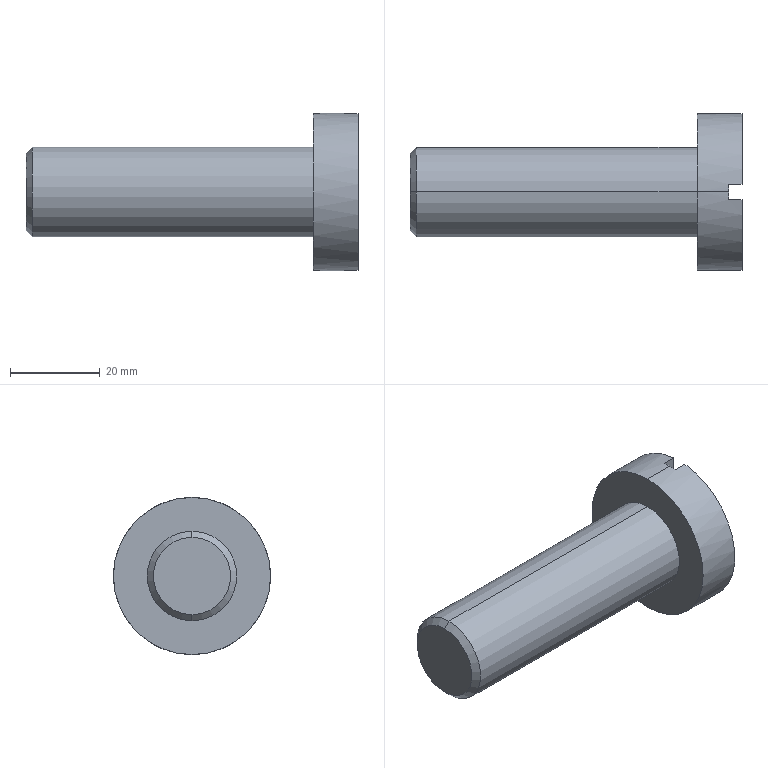Part | SolidWorks | features ICE 3, Extrusion 1, StudWizard 1 | 1 solid | 13 faces | box 74 x 35 x 35 mm | volume 29304 mm3 | plane 7 | cylinder 4 | cone 2 | commonest cylinder face diameters 20 x2 35 x2
STEP:
#1=CARTESIAN_POINT('',(-64.,0.,-8.626));
#2=VERTEX_POINT('',#1);
#3=CARTESIAN_POINT('',(-64.,0.,8.626));
#4=VERTEX_POINT('',#3);
#5=CARTESIAN_POINT('',(-64.,0.,0.));
#6=DIRECTION('',(1.,0.,0.));
#7=DIRECTION('',(0.,0.,-1.));
#8=AXIS2_PLACEMENT_3D('',#5,#6,#7);
#9=CIRCLE('',#8,8.626);
#10=EDGE_CURVE('',#2,#4,#9,.T.);
#11=ORIENTED_EDGE('',*,*,#10,.T.);
#12=CARTESIAN_POINT('',(-62.626,0.,10.));
#13=VERTEX_POINT('',#12);
#14=CARTESIAN_POINT('',(-64.,0.,8.626));
#15=DIRECTION('',(0.7071,0.,0.7071));
#16=VECTOR('',#15,1000.);
#17=LINE('',#14,#16);
#18=EDGE_CURVE('',#4,#13,#17,.T.);
#19=ORIENTED_EDGE('',*,*,#18,.T.);
#20=CARTESIAN_POINT('',(-62.626,0.,-10.));
#21=VERTEX_POINT('',#20);
#22=CARTESIAN_POINT('',(-62.626,0.,0.));
#23=DIRECTION('',(1.,0.,0.));
#24=DIRECTION('',(0.,0.,-1.));
#25=AXIS2_PLACEMENT_3D('',#22,#23,#24);
#26=CIRCLE('',#25,10.);
#27=EDGE_CURVE('',#21,#13,#26,.T.);
#28=ORIENTED_EDGE('',*,*,#27,.F.);
#29=CARTESIAN_POINT('',(-64.,0.,-8.626));
#30=DIRECTION('',(0.7071,0.,-0.7071));
#31=VECTOR('',#30,1000.);
#32=LINE('',#29,#31);
#33=EDGE_CURVE('',#2,#21,#32,.T.);
#34=ORIENTED_EDGE('',*,*,#33,.F.);
#35=EDGE_LOOP('',(#11,#19,#28,#34));
#36=FACE_OUTER_BOUND('',#35,.T.);
#37=CARTESIAN_POINT('',(-64.,0.,0.));
#38=DIRECTION('',(1.,0.,0.));
#39=DIRECTION('',(0.,0.,-1.));
#40=AXIS2_PLACEMENT_3D('',#37,#38,#39);
#41=CONICAL_SURFACE('',#40,8.626,0.7854);
#42=ADVANCED_FACE('',(#36),#41,.T.);
#43=ORIENTED_EDGE('',*,*,#27,.T.);
#44=CARTESIAN_POINT('',(0.,0.,10.));
#45=VERTEX_POINT('',#44);
#46=CARTESIAN_POINT('',(-49.1,0.,10.));
#47=DIRECTION('',(1.,0.,0.));
#48=VECTOR('',#47,1000.);
#49=LINE('',#46,#48);
#50=EDGE_CURVE('',#13,#45,#49,.T.);
#51=ORIENTED_EDGE('',*,*,#50,.T.);
#52=CARTESIAN_POINT('',(0.,0.,-10.));
#53=VERTEX_POINT('',#52);
#54=CARTESIAN_POINT('',(0.,0.,0.));
#55=DIRECTION('',(-1.,0.,0.));
#56=DIRECTION('',(0.,0.,1.));
#57=AXIS2_PLACEMENT_3D('',#54,#55,#56);
#58=CIRCLE('',#57,10.);
#59=EDGE_CURVE('',#45,#53,#58,.T.);
#60=ORIENTED_EDGE('',*,*,#59,.T.);
#61=CARTESIAN_POINT('',(-49.1,0.,-10.));
#62=DIRECTION('',(1.,0.,0.));
#63=VECTOR('',#62,1000.);
#64=LINE('',#61,#63);
#65=EDGE_CURVE('',#21,#53,#64,.T.);
#66=ORIENTED_EDGE('',*,*,#65,.F.);
#67=EDGE_LOOP('',(#43,#51,#60,#66));
#68=FACE_OUTER_BOUND('',#67,.T.);
#69=CARTESIAN_POINT('',(-49.1,0.,0.));
#70=DIRECTION('',(1.,0.,0.));
#71=DIRECTION('',(0.,0.,-1.));
#72=AXIS2_PLACEMENT_3D('',#69,#70,#71);
#73=CYLINDRICAL_SURFACE('',#72,10.);
#74=ADVANCED_FACE('',(#68),#73,.T.);
#75=CARTESIAN_POINT('',(7.,0.,-17.5));
#76=VERTEX_POINT('',#75);
#77=CARTESIAN_POINT('',(7.,1.75,-17.412));
#78=VERTEX_POINT('',#77);
#79=CARTESIAN_POINT('',(7.,0.,0.));
#80=DIRECTION('',(1.,0.,0.));
#81=DIRECTION('',(0.,0.,-1.));
#82=AXIS2_PLACEMENT_3D('',#79,#80,#81);
#83=CIRCLE('',#82,17.5);
#84=EDGE_CURVE('',#76,#78,#83,.T.);
#85=ORIENTED_EDGE('',*,*,#84,.F.);
#86=CARTESIAN_POINT('',(0.,0.,-17.5));
#87=VERTEX_POINT('',#86);
#88=CARTESIAN_POINT('',(10.,0.,-17.5));
#89=DIRECTION('',(-1.,0.,0.));
#90=VECTOR('',#89,1000.);
#91=LINE('',#88,#90);
#92=EDGE_CURVE('',#76,#87,#91,.T.);
#93=ORIENTED_EDGE('',*,*,#92,.T.);
#94=CARTESIAN_POINT('',(0.,0.,17.5));
#95=VERTEX_POINT('',#94);
#96=CARTESIAN_POINT('',(0.,0.,0.));
#97=DIRECTION('',(1.,0.,0.));
#98=DIRECTION('',(0.,0.,-1.));
#99=AXIS2_PLACEMENT_3D('',#96,#97,#98);
#100=CIRCLE('',#99,17.5);
#101=EDGE_CURVE('',#87,#95,#100,.T.);
#102=ORIENTED_EDGE('',*,*,#101,.T.);
#103=CARTESIAN_POINT('',(7.,0.,17.5));
#104=VERTEX_POINT('',#103);
#105=CARTESIAN_POINT('',(10.,0.,17.5));
#106=DIRECTION('',(-1.,0.,0.));
#107=VECTOR('',#106,1000.);
#108=LINE('',#105,#107);
#109=EDGE_CURVE('',#104,#95,#108,.T.);
#110=ORIENTED_EDGE('',*,*,#109,.F.);
#111=CARTESIAN_POINT('',(7.,1.75,17.412));
#112=VERTEX_POINT('',#111);
#113=CARTESIAN_POINT('',(7.,0.,0.));
#114=DIRECTION('',(1.,0.,0.));
#115=DIRECTION('',(0.,0.,-1.));
#116=AXIS2_PLACEMENT_3D('',#113,#114,#115);
#117=CIRCLE('',#116,17.5);
#118=EDGE_CURVE('',#112,#104,#117,.T.);
#119=ORIENTED_EDGE('',*,*,#118,.F.);
#120=CARTESIAN_POINT('',(10.,1.75,17.412));
#121=VERTEX_POINT('',#120);
#122=CARTESIAN_POINT('',(10.,1.75,17.412));
#123=DIRECTION('',(1.,0.,0.));
#124=VECTOR('',#123,1000.);
#125=LINE('',#122,#124);
#126=EDGE_CURVE('',#112,#121,#125,.T.);
#127=ORIENTED_EDGE('',*,*,#126,.T.);
#128=CARTESIAN_POINT('',(10.,1.75,-17.412));
#129=VERTEX_POINT('',#128);
#130=CARTESIAN_POINT('',(10.,0.,0.));
#131=DIRECTION('',(1.,0.,0.));
#132=DIRECTION('',(0.,0.,-1.));
#133=AXIS2_PLACEMENT_3D('',#130,#131,#132);
#134=CIRCLE('',#133,17.5);
#135=EDGE_CURVE('',#129,#121,#134,.T.);
#136=ORIENTED_EDGE('',*,*,#135,.F.);
#137=CARTESIAN_POINT('',(10.,1.75,-17.412));
#138=DIRECTION('',(-1.,0.,0.));
#139=VECTOR('',#138,1000.);
#140=LINE('',#137,#139);
#141=EDGE_CURVE('',#129,#78,#140,.T.);
#142=ORIENTED_EDGE('',*,*,#141,.T.);
#143=EDGE_LOOP('',(#85,#93,#102,#110,#119,#127,#136,#142));
#144=FACE_OUTER_BOUND('',#143,.T.);
#145=CARTESIAN_POINT('',(10.,0.,0.));
#146=DIRECTION('',(-1.,0.,0.));
#147=DIRECTION('',(0.,0.,1.));
#148=AXIS2_PLACEMENT_3D('',#145,#146,#147);
#149=CYLINDRICAL_SURFACE('',#148,17.5);
#150=ADVANCED_FACE('',(#144),#149,.T.);
#151=CARTESIAN_POINT('',(10.,-1.75,17.412));
#152=VERTEX_POINT('',#151);
#153=CARTESIAN_POINT('',(10.,-1.75,-17.412));
#154=VERTEX_POINT('',#153);
#155=CARTESIAN_POINT('',(10.,-1.75,0.));
#156=DIRECTION('',(0.,0.,-1.));
#157=VECTOR('',#156,1000.);
#158=LINE('',#155,#157);
#159=EDGE_CURVE('',#152,#154,#158,.T.);
#160=ORIENTED_EDGE('',*,*,#159,.F.);
#161=CARTESIAN_POINT('',(10.,0.,0.));
#162=DIRECTION('',(1.,0.,0.));
#163=DIRECTION('',(0.,0.,-1.));
#164=AXIS2_PLACEMENT_3D('',#161,#162,#163);
#165=CIRCLE('',#164,17.5);
#166=EDGE_CURVE('',#152,#154,#165,.T.);
#167=ORIENTED_EDGE('',*,*,#166,.T.);
#168=EDGE_LOOP('',(#160,#167));
#169=FACE_OUTER_BOUND('',#168,.T.);
#170=CARTESIAN_POINT('',(10.,0.,0.));
#171=DIRECTION('',(1.,0.,0.));
#172=DIRECTION('',(0.,0.,-1.));
#173=AXIS2_PLACEMENT_3D('',#170,#171,#172);
#174=PLANE('',#173);
#175=ADVANCED_FACE('',(#169),#174,.T.);
#176=ORIENTED_EDGE('',*,*,#92,.F.);
#177=CARTESIAN_POINT('',(7.,-1.75,-17.412));
#178=VERTEX_POINT('',#177);
#179=CARTESIAN_POINT('',(7.,0.,0.));
#180=DIRECTION('',(1.,0.,0.));
#181=DIRECTION('',(0.,0.,-1.));
#182=AXIS2_PLACEMENT_3D('',#179,#180,#181);
#183=CIRCLE('',#182,17.5);
#184=EDGE_CURVE('',#178,#76,#183,.T.);
#185=ORIENTED_EDGE('',*,*,#184,.F.);
#186=CARTESIAN_POINT('',(10.,-1.75,-17.412));
#187=DIRECTION('',(1.,0.,0.));
#188=VECTOR('',#187,1000.);
#189=LINE('',#186,#188);
#190=EDGE_CURVE('',#178,#154,#189,.T.);
#191=ORIENTED_EDGE('',*,*,#190,.T.);
#192=ORIENTED_EDGE('',*,*,#166,.F.);
#193=CARTESIAN_POINT('',(7.,-1.75,17.412));
#194=VERTEX_POINT('',#193);
#195=CARTESIAN_POINT('',(10.,-1.75,17.412));
#196=DIRECTION('',(-1.,0.,0.));
#197=VECTOR('',#196,1000.);
#198=LINE('',#195,#197);
#199=EDGE_CURVE('',#152,#194,#198,.T.);
#200=ORIENTED_EDGE('',*,*,#199,.T.);
#201=CARTESIAN_POINT('',(7.,0.,0.));
#202=DIRECTION('',(1.,0.,0.));
#203=DIRECTION('',(0.,0.,-1.));
#204=AXIS2_PLACEMENT_3D('',#201,#202,#203);
#205=CIRCLE('',#204,17.5);
#206=EDGE_CURVE('',#104,#194,#205,.T.);
#207=ORIENTED_EDGE('',*,*,#206,.F.);
#208=ORIENTED_EDGE('',*,*,#109,.T.);
#209=CARTESIAN_POINT('',(0.,0.,0.));
#210=DIRECTION('',(1.,0.,0.));
#211=DIRECTION('',(0.,0.,-1.));
#212=AXIS2_PLACEMENT_3D('',#209,#210,#211);
#213=CIRCLE('',#212,17.5);
#214=EDGE_CURVE('',#95,#87,#213,.T.);
#215=ORIENTED_EDGE('',*,*,#214,.T.);
#216=EDGE_LOOP('',(#176,#185,#191,#192,#200,#207,#208,#215));
#217=FACE_OUTER_BOUND('',#216,.T.);
#218=CARTESIAN_POINT('',(10.,0.,0.));
#219=DIRECTION('',(-1.,0.,0.));
#220=DIRECTION('',(0.,0.,1.));
#221=AXIS2_PLACEMENT_3D('',#218,#219,#220);
#222=CYLINDRICAL_SURFACE('',#221,17.5);
#223=ADVANCED_FACE('',(#217),#222,.T.);
#224=CARTESIAN_POINT('',(10.,1.75,0.));
#225=DIRECTION('',(0.,0.,1.));
#226=VECTOR('',#225,1000.);
#227=LINE('',#224,#226);
#228=EDGE_CURVE('',#129,#121,#227,.T.);
#229=ORIENTED_EDGE('',*,*,#228,.F.);
#230=ORIENTED_EDGE('',*,*,#135,.T.);
#231=EDGE_LOOP('',(#229,#230));
#232=FACE_OUTER_BOUND('',#231,.T.);
#233=CARTESIAN_POINT('',(10.,0.,0.));
#234=DIRECTION('',(1.,0.,0.));
#235=DIRECTION('',(0.,0.,-1.));
#236=AXIS2_PLACEMENT_3D('',#233,#234,#235);
#237=PLANE('',#236);
#238=ADVANCED_FACE('',(#232),#237,.T.);
#239=CARTESIAN_POINT('',(0.,0.,0.));
#240=DIRECTION('',(-1.,0.,0.));
#241=DIRECTION('',(0.,0.,1.));
#242=AXIS2_PLACEMENT_3D('',#239,#240,#241);
#243=CIRCLE('',#242,10.);
#244=EDGE_CURVE('',#53,#45,#243,.T.);
#245=ORIENTED_EDGE('',*,*,#244,.F.);
#246=ORIENTED_EDGE('',*,*,#59,.F.);
#247=EDGE_LOOP('',(#245,#246));
#248=FACE_BOUND('',#247,.T.);
#249=ORIENTED_EDGE('',*,*,#214,.F.);
#250=ORIENTED_EDGE('',*,*,#101,.F.);
#251=EDGE_LOOP('',(#249,#250));
#252=FACE_OUTER_BOUND('',#251,.T.);
#253=CARTESIAN_POINT('',(0.,0.,0.));
#254=DIRECTION('',(1.,0.,0.));
#255=DIRECTION('',(0.,0.,-1.));
#256=AXIS2_PLACEMENT_3D('',#253,#254,#255);
#257=PLANE('',#256);
#258=ADVANCED_FACE('',(#248,#252),#257,.F.);
#259=ORIENTED_EDGE('',*,*,#118,.T.);
#260=ORIENTED_EDGE('',*,*,#206,.T.);
#261=CARTESIAN_POINT('',(7.,-1.75,20.));
#262=DIRECTION('',(0.,0.,-1.));
#263=VECTOR('',#262,1000.);
#264=LINE('',#261,#263);
#265=EDGE_CURVE('',#194,#178,#264,.T.);
#266=ORIENTED_EDGE('',*,*,#265,.T.);
#267=ORIENTED_EDGE('',*,*,#184,.T.);
#268=ORIENTED_EDGE('',*,*,#84,.T.);
#269=CARTESIAN_POINT('',(7.,1.75,20.));
#270=DIRECTION('',(0.,0.,1.));
#271=VECTOR('',#270,1000.);
#272=LINE('',#269,#271);
#273=EDGE_CURVE('',#78,#112,#272,.T.);
#274=ORIENTED_EDGE('',*,*,#273,.T.);
#275=EDGE_LOOP('',(#259,#260,#266,#267,#268,#274));
#276=FACE_OUTER_BOUND('',#275,.T.);
#277=CARTESIAN_POINT('',(7.,0.,0.));
#278=DIRECTION('',(1.,0.,0.));
#279=DIRECTION('',(0.,0.,-1.));
#280=AXIS2_PLACEMENT_3D('',#277,#278,#279);
#281=PLANE('',#280);
#282=ADVANCED_FACE('',(#276),#281,.T.);
#283=ORIENTED_EDGE('',*,*,#159,.T.);
#284=ORIENTED_EDGE('',*,*,#190,.F.);
#285=ORIENTED_EDGE('',*,*,#265,.F.);
#286=ORIENTED_EDGE('',*,*,#199,.F.);
#287=EDGE_LOOP('',(#283,#284,#285,#286));
#288=FACE_OUTER_BOUND('',#287,.T.);
#289=CARTESIAN_POINT('',(7.,-1.75,20.));
#290=DIRECTION('',(0.,-1.,0.));
#291=DIRECTION('',(0.,0.,-1.));
#292=AXIS2_PLACEMENT_3D('',#289,#290,#291);
#293=PLANE('',#292);
#294=ADVANCED_FACE('',(#288),#293,.F.);
#295=ORIENTED_EDGE('',*,*,#228,.T.);
#296=ORIENTED_EDGE('',*,*,#126,.F.);
#297=ORIENTED_EDGE('',*,*,#273,.F.);
#298=ORIENTED_EDGE('',*,*,#141,.F.);
#299=EDGE_LOOP('',(#295,#296,#297,#298));
#300=FACE_OUTER_BOUND('',#299,.T.);
#301=CARTESIAN_POINT('',(7.,1.75,20.));
#302=DIRECTION('',(0.,1.,0.));
#303=DIRECTION('',(0.,0.,1.));
#304=AXIS2_PLACEMENT_3D('',#301,#302,#303);
#305=PLANE('',#304);
#306=ADVANCED_FACE('',(#300),#305,.F.);
#307=ORIENTED_EDGE('',*,*,#50,.F.);
#308=CARTESIAN_POINT('',(-62.626,0.,0.));
#309=DIRECTION('',(1.,0.,0.));
#310=DIRECTION('',(0.,0.,-1.));
#311=AXIS2_PLACEMENT_3D('',#308,#309,#310);
#312=CIRCLE('',#311,10.);
#313=EDGE_CURVE('',#13,#21,#312,.T.);
#314=ORIENTED_EDGE('',*,*,#313,.T.);
#315=ORIENTED_EDGE('',*,*,#65,.T.);
#316=ORIENTED_EDGE('',*,*,#244,.T.);
#317=EDGE_LOOP('',(#307,#314,#315,#316));
#318=FACE_OUTER_BOUND('',#317,.T.);
#319=CARTESIAN_POINT('',(-49.1,0.,0.));
#320=DIRECTION('',(1.,0.,0.));
#321=DIRECTION('',(0.,0.,-1.));
#322=AXIS2_PLACEMENT_3D('',#319,#320,#321);
#323=CYLINDRICAL_SURFACE('',#322,10.);
#324=ADVANCED_FACE('',(#318),#323,.T.);
#325=ORIENTED_EDGE('',*,*,#18,.F.);
#326=CARTESIAN_POINT('',(-64.,0.,0.));
#327=DIRECTION('',(1.,0.,0.));
#328=DIRECTION('',(0.,0.,-1.));
#329=AXIS2_PLACEMENT_3D('',#326,#327,#328);
#330=CIRCLE('',#329,8.626);
#331=EDGE_CURVE('',#4,#2,#330,.T.);
#332=ORIENTED_EDGE('',*,*,#331,.T.);
#333=ORIENTED_EDGE('',*,*,#33,.T.);
#334=ORIENTED_EDGE('',*,*,#313,.F.);
#335=EDGE_LOOP('',(#325,#332,#333,#334));
#336=FACE_OUTER_BOUND('',#335,.T.);
#337=CARTESIAN_POINT('',(-64.,0.,0.));
#338=DIRECTION('',(1.,0.,0.));
#339=DIRECTION('',(0.,0.,-1.));
#340=AXIS2_PLACEMENT_3D('',#337,#338,#339);
#341=CONICAL_SURFACE('',#340,8.626,0.7854);
#342=ADVANCED_FACE('',(#336),#341,.T.);
#343=ORIENTED_EDGE('',*,*,#10,.F.);
#344=ORIENTED_EDGE('',*,*,#331,.F.);
#345=EDGE_LOOP('',(#343,#344));
#346=FACE_OUTER_BOUND('',#345,.T.);
#347=CARTESIAN_POINT('',(-64.,0.,0.));
#348=DIRECTION('',(-1.,0.,0.));
#349=DIRECTION('',(0.,0.,1.));
#350=AXIS2_PLACEMENT_3D('',#347,#348,#349);
#351=PLANE('',#350);
#352=ADVANCED_FACE('',(#346),#351,.T.);
#353=CLOSED_SHELL('',(#42,#74,#150,#175,#223,#238,#258,#282,#294,#306,#324,#342,#352));
#354=MANIFOLD_SOLID_BREP('',#353);
#355=CARTESIAN_POINT('',(0.,0.,0.));
#356=DIRECTION('',(0.,0.,1.));
#357=DIRECTION('',(1.,0.,0.));
#358=AXIS2_PLACEMENT_3D('',#355,#356,#357);
#359=(LENGTH_UNIT()NAMED_UNIT(*)SI_UNIT(.MILLI.,.METRE.));
#360=UNCERTAINTY_MEASURE_WITH_UNIT(LENGTH_MEASURE(0.00001),#359,'','');
#361=(NAMED_UNIT(*)PLANE_ANGLE_UNIT()SI_UNIT($,.RADIAN.));
#362=(NAMED_UNIT(*)SI_UNIT($,.STERADIAN.)SOLID_ANGLE_UNIT());
#363=(GEOMETRIC_REPRESENTATION_CONTEXT(3)GLOBAL_UNCERTAINTY_ASSIGNED_CONTEXT((#360))GLOBAL_UNIT_ASSIGNED_CONTEXT((#359,#361,#362))REPRESENTATION_CONTEXT('',''));
#364=ADVANCED_BREP_SHAPE_REPRESENTATION('',(#354,#358),#363);